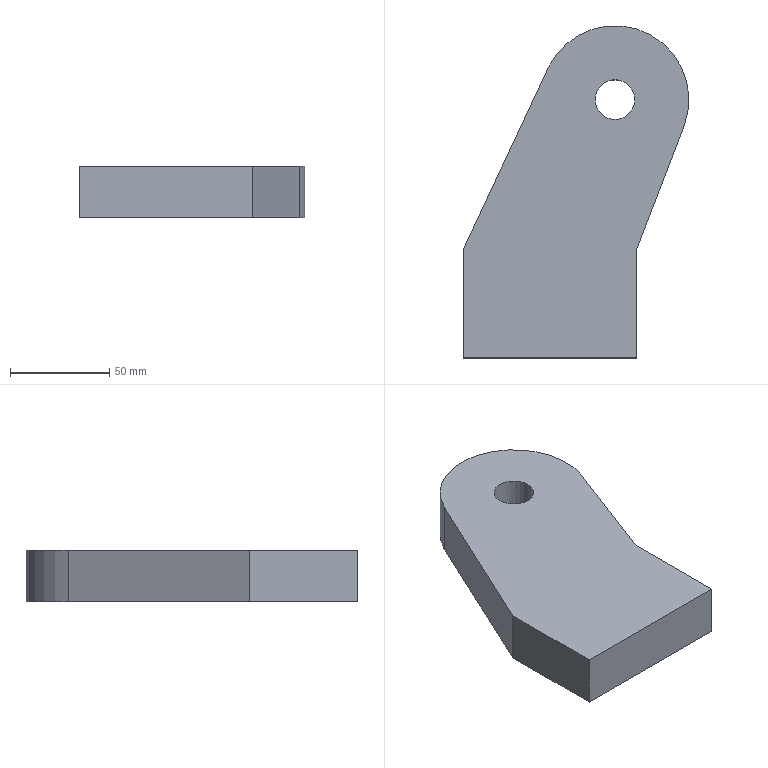Part | NX | features 底座(默认<按焊接>) 2 | 1 solid | 9 faces | box 113.6 x 167.23 x 26 mm | volume 337496 mm3 | plane 7 | cylinder 2 | commonest cylinder face diameters 20 x1 74.46 x1
STEP:
#1=CARTESIAN_POINT('',(1430.091,683.975,-665.));
#2=VERTEX_POINT('',#1);
#3=CARTESIAN_POINT('',(1361.609,713.087,-665.));
#4=VERTEX_POINT('',#3);
#5=CARTESIAN_POINT('',(1395.335,697.32,-665.));
#6=DIRECTION('',(0.,0.,1.));
#7=DIRECTION('',(1.,0.,0.));
#8=AXIS2_PLACEMENT_3D('',#5,#6,#7);
#9=CIRCLE('',#8,37.23);
#10=EDGE_CURVE('',#2,#4,#9,.T.);
#11=ORIENTED_EDGE('',*,*,#10,.F.);
#12=CARTESIAN_POINT('',(1406.245,621.87,-665.));
#13=VERTEX_POINT('',#12);
#14=CARTESIAN_POINT('',(1430.091,683.975,-665.));
#15=DIRECTION('',(0.3584,0.9335,0.));
#16=VECTOR('',#15,1000.);
#17=LINE('',#14,#16);
#18=EDGE_CURVE('',#13,#2,#17,.T.);
#19=ORIENTED_EDGE('',*,*,#18,.F.);
#20=CARTESIAN_POINT('',(1406.245,567.32,-665.));
#21=VERTEX_POINT('',#20);
#22=CARTESIAN_POINT('',(1406.245,621.87,-665.));
#23=DIRECTION('',(0.,1.,0.));
#24=VECTOR('',#23,1000.);
#25=LINE('',#22,#24);
#26=EDGE_CURVE('',#21,#13,#25,.T.);
#27=ORIENTED_EDGE('',*,*,#26,.F.);
#28=CARTESIAN_POINT('',(1318.965,567.32,-665.));
#29=VERTEX_POINT('',#28);
#30=CARTESIAN_POINT('',(1406.245,567.32,-665.));
#31=DIRECTION('',(1.,0.,0.));
#32=VECTOR('',#31,1000.);
#33=LINE('',#30,#32);
#34=EDGE_CURVE('',#29,#21,#33,.T.);
#35=ORIENTED_EDGE('',*,*,#34,.F.);
#36=CARTESIAN_POINT('',(1318.965,621.87,-665.));
#37=VERTEX_POINT('',#36);
#38=CARTESIAN_POINT('',(1318.965,621.87,-665.));
#39=DIRECTION('',(0.,-1.,0.));
#40=VECTOR('',#39,1000.);
#41=LINE('',#38,#40);
#42=EDGE_CURVE('',#37,#29,#41,.T.);
#43=ORIENTED_EDGE('',*,*,#42,.F.);
#44=CARTESIAN_POINT('',(1361.609,713.087,-665.));
#45=DIRECTION('',(-0.4235,-0.9059,0.));
#46=VECTOR('',#45,1000.);
#47=LINE('',#44,#46);
#48=EDGE_CURVE('',#4,#37,#47,.T.);
#49=ORIENTED_EDGE('',*,*,#48,.F.);
#50=EDGE_LOOP('',(#11,#19,#27,#35,#43,#49));
#51=FACE_BOUND('',#50,.T.);
#52=CARTESIAN_POINT('',(1405.335,697.32,-665.));
#53=VERTEX_POINT('',#52);
#54=CARTESIAN_POINT('',(1395.335,697.32,-665.));
#55=DIRECTION('',(0.,0.,1.));
#56=DIRECTION('',(1.,0.,0.));
#57=AXIS2_PLACEMENT_3D('',#54,#55,#56);
#58=CIRCLE('',#57,10.);
#59=EDGE_CURVE('',#53,#53,#58,.T.);
#60=ORIENTED_EDGE('',*,*,#59,.T.);
#61=EDGE_LOOP('',(#60));
#62=FACE_BOUND('',#61,.T.);
#63=CARTESIAN_POINT('',(1395.335,697.32,-665.));
#64=DIRECTION('',(0.,0.,-1.));
#65=DIRECTION('',(1.,0.,0.));
#66=AXIS2_PLACEMENT_3D('',#63,#64,#65);
#67=PLANE('',#66);
#68=ADVANCED_FACE('',(#51,#62),#67,.T.);
#69=CARTESIAN_POINT('',(1430.091,683.975,-639.));
#70=VERTEX_POINT('',#69);
#71=CARTESIAN_POINT('',(1361.609,713.087,-639.));
#72=VERTEX_POINT('',#71);
#73=CARTESIAN_POINT('',(1395.335,697.32,-639.));
#74=DIRECTION('',(0.,0.,1.));
#75=DIRECTION('',(1.,0.,0.));
#76=AXIS2_PLACEMENT_3D('',#73,#74,#75);
#77=CIRCLE('',#76,37.23);
#78=EDGE_CURVE('',#70,#72,#77,.T.);
#79=ORIENTED_EDGE('',*,*,#78,.T.);
#80=CARTESIAN_POINT('',(1318.965,621.87,-639.));
#81=VERTEX_POINT('',#80);
#82=CARTESIAN_POINT('',(1361.609,713.087,-639.));
#83=DIRECTION('',(-0.4235,-0.9059,0.));
#84=VECTOR('',#83,1000.);
#85=LINE('',#82,#84);
#86=EDGE_CURVE('',#72,#81,#85,.T.);
#87=ORIENTED_EDGE('',*,*,#86,.T.);
#88=CARTESIAN_POINT('',(1318.965,567.32,-639.));
#89=VERTEX_POINT('',#88);
#90=CARTESIAN_POINT('',(1318.965,621.87,-639.));
#91=DIRECTION('',(0.,-1.,0.));
#92=VECTOR('',#91,1000.);
#93=LINE('',#90,#92);
#94=EDGE_CURVE('',#81,#89,#93,.T.);
#95=ORIENTED_EDGE('',*,*,#94,.T.);
#96=CARTESIAN_POINT('',(1406.245,567.32,-639.));
#97=VERTEX_POINT('',#96);
#98=CARTESIAN_POINT('',(1406.245,567.32,-639.));
#99=DIRECTION('',(1.,0.,0.));
#100=VECTOR('',#99,1000.);
#101=LINE('',#98,#100);
#102=EDGE_CURVE('',#89,#97,#101,.T.);
#103=ORIENTED_EDGE('',*,*,#102,.T.);
#104=CARTESIAN_POINT('',(1406.245,621.87,-639.));
#105=VERTEX_POINT('',#104);
#106=CARTESIAN_POINT('',(1406.245,621.87,-639.));
#107=DIRECTION('',(0.,1.,0.));
#108=VECTOR('',#107,1000.);
#109=LINE('',#106,#108);
#110=EDGE_CURVE('',#97,#105,#109,.T.);
#111=ORIENTED_EDGE('',*,*,#110,.T.);
#112=CARTESIAN_POINT('',(1430.091,683.975,-639.));
#113=DIRECTION('',(0.3584,0.9335,0.));
#114=VECTOR('',#113,1000.);
#115=LINE('',#112,#114);
#116=EDGE_CURVE('',#105,#70,#115,.T.);
#117=ORIENTED_EDGE('',*,*,#116,.T.);
#118=EDGE_LOOP('',(#79,#87,#95,#103,#111,#117));
#119=FACE_BOUND('',#118,.T.);
#120=CARTESIAN_POINT('',(1405.335,697.32,-639.));
#121=VERTEX_POINT('',#120);
#122=CARTESIAN_POINT('',(1395.335,697.32,-639.));
#123=DIRECTION('',(0.,0.,1.));
#124=DIRECTION('',(1.,0.,0.));
#125=AXIS2_PLACEMENT_3D('',#122,#123,#124);
#126=CIRCLE('',#125,10.);
#127=EDGE_CURVE('',#121,#121,#126,.T.);
#128=ORIENTED_EDGE('',*,*,#127,.F.);
#129=EDGE_LOOP('',(#128));
#130=FACE_BOUND('',#129,.T.);
#131=CARTESIAN_POINT('',(1395.335,697.32,-639.));
#132=DIRECTION('',(0.,0.,-1.));
#133=DIRECTION('',(1.,0.,0.));
#134=AXIS2_PLACEMENT_3D('',#131,#132,#133);
#135=PLANE('',#134);
#136=ADVANCED_FACE('',(#119,#130),#135,.F.);
#137=ORIENTED_EDGE('',*,*,#78,.F.);
#138=CARTESIAN_POINT('',(1430.091,683.975,-665.));
#139=DIRECTION('',(0.,0.,1.));
#140=VECTOR('',#139,1000.);
#141=LINE('',#138,#140);
#142=EDGE_CURVE('',#2,#70,#141,.T.);
#143=ORIENTED_EDGE('',*,*,#142,.F.);
#144=ORIENTED_EDGE('',*,*,#10,.T.);
#145=CARTESIAN_POINT('',(1361.609,713.087,-665.));
#146=DIRECTION('',(0.,0.,1.));
#147=VECTOR('',#146,1000.);
#148=LINE('',#145,#147);
#149=EDGE_CURVE('',#4,#72,#148,.T.);
#150=ORIENTED_EDGE('',*,*,#149,.T.);
#151=EDGE_LOOP('',(#137,#143,#144,#150));
#152=FACE_BOUND('',#151,.T.);
#153=CARTESIAN_POINT('',(1395.335,697.32,-665.));
#154=DIRECTION('',(0.,0.,1.));
#155=DIRECTION('',(-1.,0.,0.));
#156=AXIS2_PLACEMENT_3D('',#153,#154,#155);
#157=CYLINDRICAL_SURFACE('',#156,37.23);
#158=ADVANCED_FACE('',(#152),#157,.T.);
#159=ORIENTED_EDGE('',*,*,#86,.F.);
#160=ORIENTED_EDGE('',*,*,#149,.F.);
#161=ORIENTED_EDGE('',*,*,#48,.T.);
#162=CARTESIAN_POINT('',(1318.965,621.87,-665.));
#163=DIRECTION('',(0.,0.,1.));
#164=VECTOR('',#163,1000.);
#165=LINE('',#162,#164);
#166=EDGE_CURVE('',#37,#81,#165,.T.);
#167=ORIENTED_EDGE('',*,*,#166,.T.);
#168=EDGE_LOOP('',(#159,#160,#161,#167));
#169=FACE_BOUND('',#168,.T.);
#170=CARTESIAN_POINT('',(1361.609,713.087,-665.));
#171=DIRECTION('',(0.9059,-0.4235,0.));
#172=DIRECTION('',(0.4235,0.9059,0.));
#173=AXIS2_PLACEMENT_3D('',#170,#171,#172);
#174=PLANE('',#173);
#175=ADVANCED_FACE('',(#169),#174,.F.);
#176=ORIENTED_EDGE('',*,*,#94,.F.);
#177=ORIENTED_EDGE('',*,*,#166,.F.);
#178=ORIENTED_EDGE('',*,*,#42,.T.);
#179=CARTESIAN_POINT('',(1318.965,567.32,-665.));
#180=DIRECTION('',(0.,0.,1.));
#181=VECTOR('',#180,1000.);
#182=LINE('',#179,#181);
#183=EDGE_CURVE('',#29,#89,#182,.T.);
#184=ORIENTED_EDGE('',*,*,#183,.T.);
#185=EDGE_LOOP('',(#176,#177,#178,#184));
#186=FACE_BOUND('',#185,.T.);
#187=CARTESIAN_POINT('',(1318.965,621.87,-665.));
#188=DIRECTION('',(1.,0.,0.));
#189=DIRECTION('',(0.,0.,1.));
#190=AXIS2_PLACEMENT_3D('',#187,#188,#189);
#191=PLANE('',#190);
#192=ADVANCED_FACE('',(#186),#191,.F.);
#193=ORIENTED_EDGE('',*,*,#102,.F.);
#194=ORIENTED_EDGE('',*,*,#183,.F.);
#195=ORIENTED_EDGE('',*,*,#34,.T.);
#196=CARTESIAN_POINT('',(1406.245,567.32,-665.));
#197=DIRECTION('',(0.,0.,1.));
#198=VECTOR('',#197,1000.);
#199=LINE('',#196,#198);
#200=EDGE_CURVE('',#21,#97,#199,.T.);
#201=ORIENTED_EDGE('',*,*,#200,.T.);
#202=EDGE_LOOP('',(#193,#194,#195,#201));
#203=FACE_BOUND('',#202,.T.);
#204=CARTESIAN_POINT('',(1406.245,567.32,-665.));
#205=DIRECTION('',(0.,1.,0.));
#206=DIRECTION('',(-1.,0.,0.));
#207=AXIS2_PLACEMENT_3D('',#204,#205,#206);
#208=PLANE('',#207);
#209=ADVANCED_FACE('',(#203),#208,.F.);
#210=ORIENTED_EDGE('',*,*,#110,.F.);
#211=ORIENTED_EDGE('',*,*,#200,.F.);
#212=ORIENTED_EDGE('',*,*,#26,.T.);
#213=CARTESIAN_POINT('',(1406.245,621.87,-665.));
#214=DIRECTION('',(0.,0.,1.));
#215=VECTOR('',#214,1000.);
#216=LINE('',#213,#215);
#217=EDGE_CURVE('',#13,#105,#216,.T.);
#218=ORIENTED_EDGE('',*,*,#217,.T.);
#219=EDGE_LOOP('',(#210,#211,#212,#218));
#220=FACE_BOUND('',#219,.T.);
#221=CARTESIAN_POINT('',(1406.245,621.87,-665.));
#222=DIRECTION('',(-1.,0.,0.));
#223=DIRECTION('',(0.,0.,-1.));
#224=AXIS2_PLACEMENT_3D('',#221,#222,#223);
#225=PLANE('',#224);
#226=ADVANCED_FACE('',(#220),#225,.F.);
#227=ORIENTED_EDGE('',*,*,#116,.F.);
#228=ORIENTED_EDGE('',*,*,#217,.F.);
#229=ORIENTED_EDGE('',*,*,#18,.T.);
#230=ORIENTED_EDGE('',*,*,#142,.T.);
#231=EDGE_LOOP('',(#227,#228,#229,#230));
#232=FACE_BOUND('',#231,.T.);
#233=CARTESIAN_POINT('',(1430.091,683.975,-665.));
#234=DIRECTION('',(-0.9335,0.3584,0.));
#235=DIRECTION('',(-0.3584,-0.9335,0.));
#236=AXIS2_PLACEMENT_3D('',#233,#234,#235);
#237=PLANE('',#236);
#238=ADVANCED_FACE('',(#232),#237,.F.);
#239=ORIENTED_EDGE('',*,*,#59,.F.);
#240=EDGE_LOOP('',(#239));
#241=FACE_BOUND('',#240,.T.);
#242=ORIENTED_EDGE('',*,*,#127,.T.);
#243=EDGE_LOOP('',(#242));
#244=FACE_BOUND('',#243,.T.);
#245=CARTESIAN_POINT('',(1395.335,697.32,-665.));
#246=DIRECTION('',(0.,0.,1.));
#247=DIRECTION('',(-1.,0.,0.));
#248=AXIS2_PLACEMENT_3D('',#245,#246,#247);
#249=CYLINDRICAL_SURFACE('',#248,10.);
#250=ADVANCED_FACE('',(#241,#244),#249,.F.);
#251=CLOSED_SHELL('',(#68,#136,#158,#175,#192,#209,#226,#238,#250));
#252=MANIFOLD_SOLID_BREP('',#251);
#253=(LENGTH_UNIT()NAMED_UNIT(*)SI_UNIT(.MILLI.,.METRE.));
#254=UNCERTAINTY_MEASURE_WITH_UNIT(LENGTH_MEASURE(0.00001),#253,'','');
#255=(NAMED_UNIT(*)PLANE_ANGLE_UNIT()SI_UNIT($,.RADIAN.));
#256=(NAMED_UNIT(*)SI_UNIT($,.STERADIAN.)SOLID_ANGLE_UNIT());
#257=(GEOMETRIC_REPRESENTATION_CONTEXT(3)GLOBAL_UNCERTAINTY_ASSIGNED_CONTEXT((#254))GLOBAL_UNIT_ASSIGNED_CONTEXT((#253,#255,#256))REPRESENTATION_CONTEXT('',''));
#258=ADVANCED_BREP_SHAPE_REPRESENTATION('',(#252),#257);